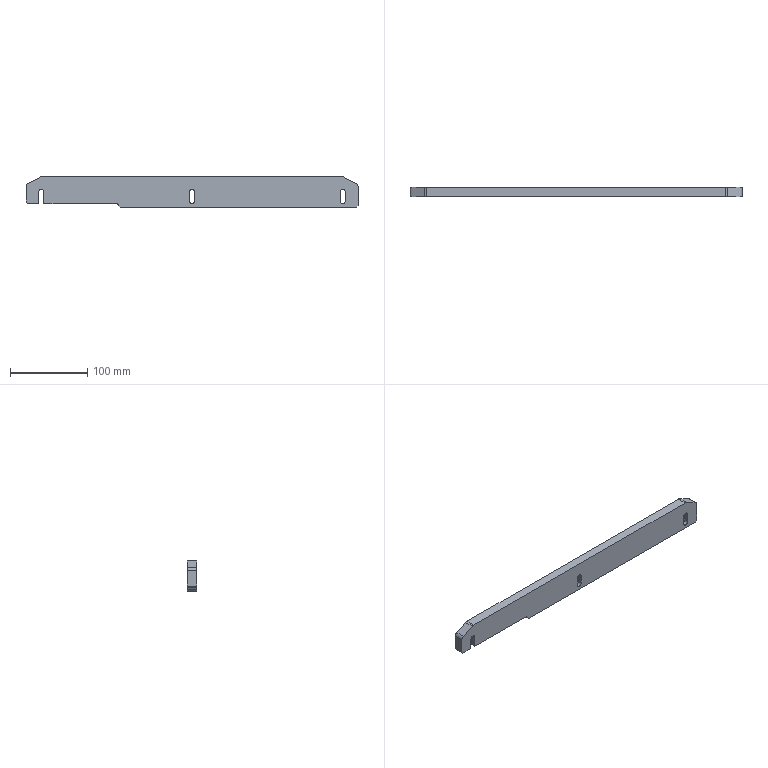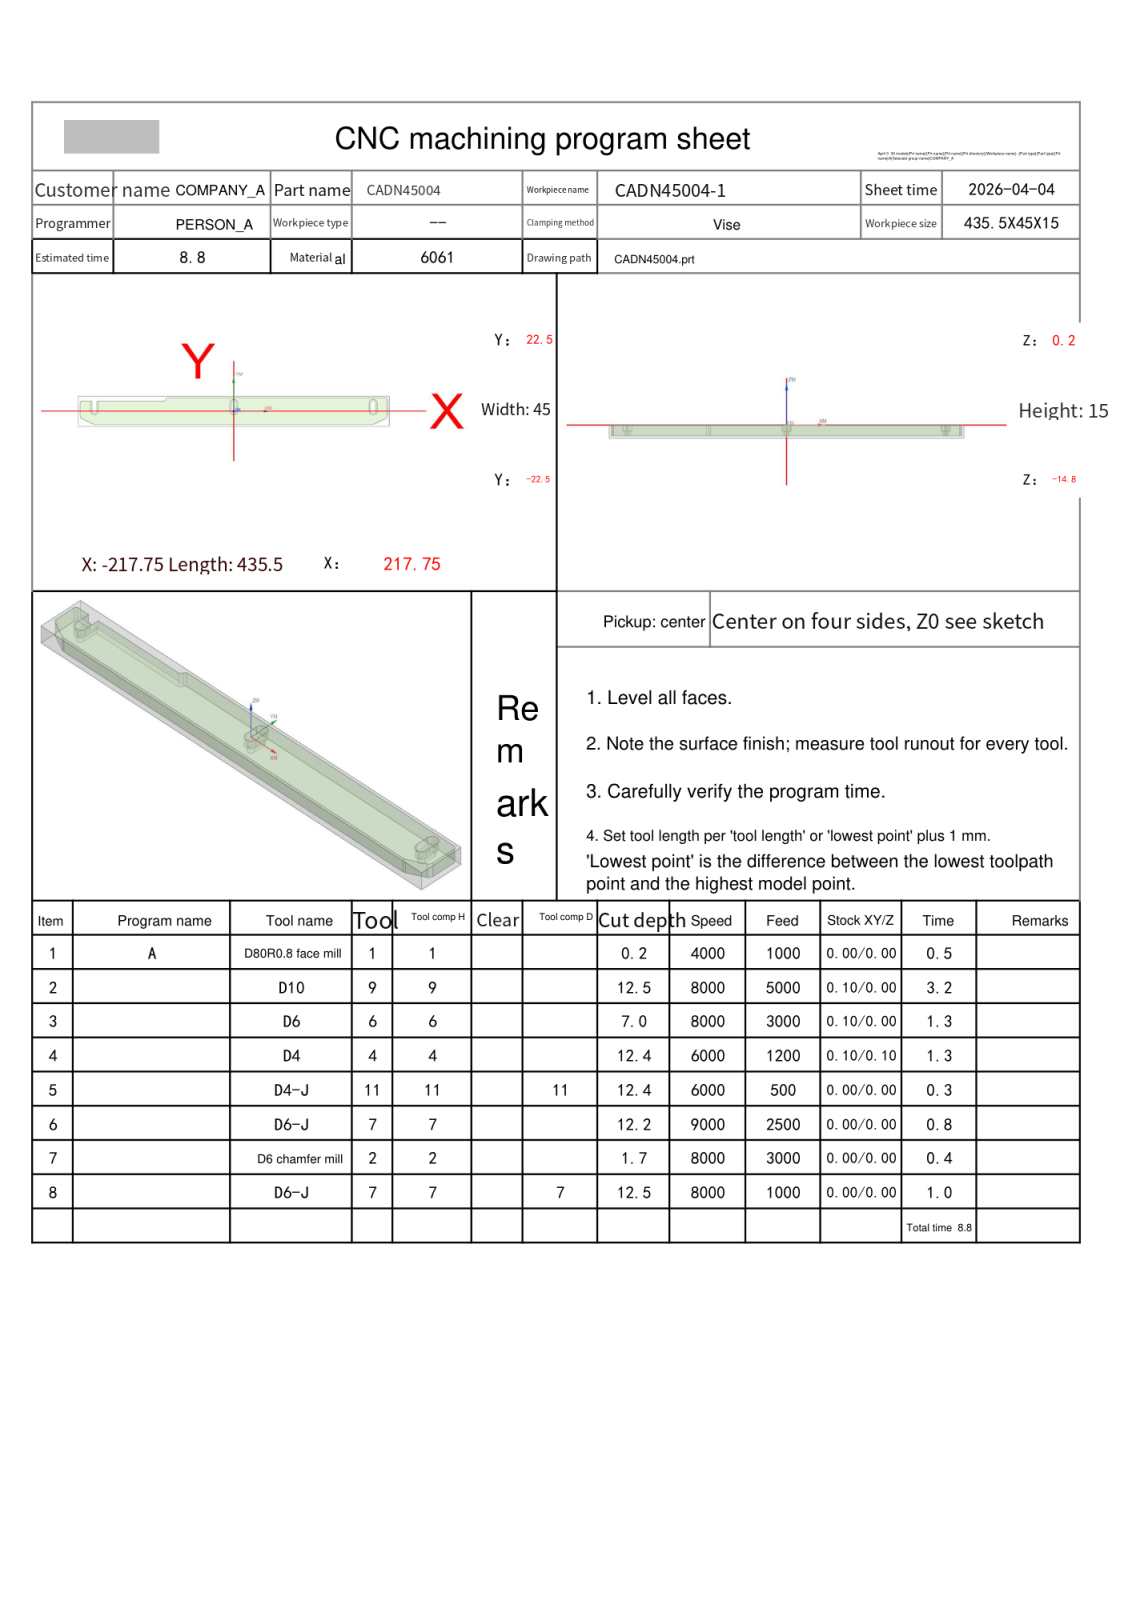NC program | NX | posted by the shop | part box 430.5 x 12 x 40 mm
Lines 1 to 1346 of 3420, first 1256 of 1344 lines:
%
O0001
(Machine time: 10.58 MIN)
(===Total Tool:7===)
(T1=D80R0.8 face mill D=80.  R=0.8  D-  H01 Z=-0.   )
(T9=D10     D=10.  R=0.   D-  H09 Z=-12.3 )
(T6=D6      D=6.   R=0.   D-  H06 Z=-6.8  )
(T4=D4      D=4.   R=0.   D-  H04 Z=-12.2 )
(T11=D4-J   D=4.   R=0.   D11 H11 Z=-12.2 )
(T7=D6-J    D=6.   R=0.   D7  H07 Z=-12.3 )
(T2=D6 chamfer mill   D=6.   R=0.   D-  H02 Z=-1.5  )
G80 G90 G17 G49 G40
G91 G28 Z0
M01
N1 T01 M06
(D80R0.8 face mill  D=80. R=0.8 H=01 ce=0.00 di=0.00)
G00 G90 G54 X260.25 Y0.0 M03 S4000
G43 H01 Z20.
M08
Z2.
G01 Z0.0 F1000.
X255.25
X-255.25
X-260.25
Z2.
G00 Z20.
G91 G28 Z0.0
M05
M09
G91 G28 Z0.0
M01
N2 T09 M06
(D10  D=10. R=0. H=09 ce=0.10 di=0.00)
G00 G90 G54 X0.0 Y-25.1 M03 S8000
G43 H09 Z20.
M08
Z.5
G01 X-194.07 Z.337 F5000.
G02 X-198.587 Y-24.034 Z.333 I0.0 J10.1
G01 X-214.767 Y-15.944 Z.318
G02 X-220.35 Y-6.91 Z.308 I4.517 J9.034
G01 Y13. Z.292
G02 X-218.856 Y16.606 Z.288 I5.1 J0.0
G01 X-216.856 Y18.606 Z.286
G02 X-213.25 Y20.1 Z.282 I3.606 J-3.606
G01 X-198.55 Z.27
G02 X-195.25 Y18.888 Z.267 I0.0 J-5.1
X-191.95 Y20.1 Z.264 I3.3 J-3.888
G01 X-99.898 Z.187
G02 X-98.856 Y21.606 Z.185 I4.648 J-2.1
G01 X-96.856 Y23.606 Z.183
G02 X-93.25 Y25.1 Z.179 I3.606 J-3.606
G01 X213.25 Z-.078
G02 X216.856 Y23.606 Z-.082 I0.0 J-5.1
G01 X218.856 Y21.606 Z-.084
G02 X220.35 Y18. Z-.087 I-3.606 J-3.606
G01 Y-6.91 Z-.108
G02 X214.767 Y-15.944 Z-.118 I-10.1 J0.0
G01 X198.587 Y-24.034 Z-.133
G02 X194.07 Y-25.1 Z-.137 I-4.517 J9.034
G01 X-194.07 Z-.463
G02 X-198.587 Y-24.034 Z-.467 I0.0 J10.1
G01 X-214.767 Y-15.944 Z-.482
G02 X-220.35 Y-6.91 Z-.492 I4.517 J9.034
G01 Y13. Z-.508
G02 X-218.856 Y16.606 Z-.512 I5.1 J0.0
G01 X-216.856 Y18.606 Z-.514
G02 X-213.25 Y20.1 Z-.518 I3.606 J-3.606
G01 X-198.55 Z-.53
G02 X-195.25 Y18.888 Z-.533 I0.0 J-5.1
X-191.95 Y20.1 Z-.536 I3.3 J-3.888
G01 X-99.898 Z-.613
G02 X-98.856 Y21.606 Z-.615 I4.648 J-2.1
G01 X-96.856 Y23.606 Z-.617
G02 X-93.25 Y25.1 Z-.621 I3.606 J-3.606
G01 X213.25 Z-.878
G02 X216.856 Y23.606 Z-.882 I0.0 J-5.1
G01 X218.856 Y21.606 Z-.884
G02 X220.35 Y18. Z-.887 I-3.606 J-3.606
G01 Y-6.91 Z-.908
G02 X214.767 Y-15.944 Z-.918 I-10.1 J0.0
G01 X198.587 Y-24.034 Z-.933
G02 X194.07 Y-25.1 Z-.937 I-4.517 J9.034
G01 X-194.07 Z-1.263
G02 X-198.587 Y-24.034 Z-1.267 I0.0 J10.1
G01 X-214.767 Y-15.944 Z-1.282
G02 X-220.35 Y-6.91 Z-1.292 I4.517 J9.034
G01 Y13. Z-1.308
G02 X-218.856 Y16.606 Z-1.312 I5.1 J0.0
G01 X-216.856 Y18.606 Z-1.314
G02 X-213.25 Y20.1 Z-1.318 I3.606 J-3.606
G01 X-198.55 Z-1.33
G02 X-195.25 Y18.888 Z-1.333 I0.0 J-5.1
X-191.95 Y20.1 Z-1.336 I3.3 J-3.888
G01 X-99.898 Z-1.413
G02 X-98.856 Y21.606 Z-1.415 I4.648 J-2.1
G01 X-96.856 Y23.606 Z-1.417
G02 X-93.25 Y25.1 Z-1.421 I3.606 J-3.606
G01 X213.25 Z-1.678
G02 X216.856 Y23.606 Z-1.682 I0.0 J-5.1
G01 X218.856 Y21.606 Z-1.684
G02 X220.35 Y18. Z-1.687 I-3.606 J-3.606
G01 Y-6.91 Z-1.708
G02 X214.767 Y-15.944 Z-1.718 I-10.1 J0.0
G01 X198.587 Y-24.034 Z-1.733
G02 X194.07 Y-25.1 Z-1.737 I-4.517 J9.034
G01 X-194.07 Z-2.063
G02 X-198.587 Y-24.034 Z-2.067 I0.0 J10.1
G01 X-214.767 Y-15.944 Z-2.082
G02 X-220.35 Y-6.91 Z-2.092 I4.517 J9.034
G01 Y13. Z-2.108
G02 X-218.856 Y16.606 Z-2.112 I5.1 J0.0
G01 X-216.856 Y18.606 Z-2.114
G02 X-213.25 Y20.1 Z-2.118 I3.606 J-3.606
G01 X-198.55 Z-2.13
G02 X-195.25 Y18.888 Z-2.133 I0.0 J-5.1
X-191.95 Y20.1 Z-2.136 I3.3 J-3.888
G01 X-99.898 Z-2.213
G02 X-98.856 Y21.606 Z-2.215 I4.648 J-2.1
G01 X-96.856 Y23.606 Z-2.217
G02 X-93.25 Y25.1 Z-2.221 I3.606 J-3.606
G01 X213.25 Z-2.478
G02 X216.856 Y23.606 Z-2.482 I0.0 J-5.1
G01 X218.856 Y21.606 Z-2.484
G02 X220.35 Y18. Z-2.487 I-3.606 J-3.606
G01 Y-6.91 Z-2.508
G02 X214.767 Y-15.944 Z-2.518 I-10.1 J0.0
G01 X198.587 Y-24.034 Z-2.533
G02 X194.07 Y-25.1 Z-2.537 I-4.517 J9.034
G01 X-194.07 Z-2.863
G02 X-198.587 Y-24.034 Z-2.867 I0.0 J10.1
G01 X-214.767 Y-15.944 Z-2.882
G02 X-220.35 Y-6.91 Z-2.892 I4.517 J9.034
G01 Y13. Z-2.908
G02 X-218.856 Y16.606 Z-2.912 I5.1 J0.0
G01 X-216.856 Y18.606 Z-2.914
G02 X-213.25 Y20.1 Z-2.918 I3.606 J-3.606
G01 X-198.55 Z-2.93
G02 X-195.25 Y18.888 Z-2.933 I0.0 J-5.1
X-191.95 Y20.1 Z-2.936 I3.3 J-3.888
G01 X-99.898 Z-3.013
G02 X-98.856 Y21.606 Z-3.015 I4.648 J-2.1
G01 X-96.856 Y23.606 Z-3.017
G02 X-93.25 Y25.1 Z-3.021 I3.606 J-3.606
G01 X213.25 Z-3.278
G02 X216.856 Y23.606 Z-3.282 I0.0 J-5.1
G01 X218.856 Y21.606 Z-3.284
G02 X220.35 Y18. Z-3.287 I-3.606 J-3.606
G01 Y-6.91 Z-3.308
G02 X214.767 Y-15.944 Z-3.318 I-10.1 J0.0
G01 X198.587 Y-24.034 Z-3.333
G02 X194.07 Y-25.1 Z-3.337 I-4.517 J9.034
G01 X-194.07 Z-3.663
G02 X-198.587 Y-24.034 Z-3.667 I0.0 J10.1
G01 X-214.767 Y-15.944 Z-3.682
G02 X-220.35 Y-6.91 Z-3.692 I4.517 J9.034
G01 Y13. Z-3.708
G02 X-218.856 Y16.606 Z-3.712 I5.1 J0.0
G01 X-216.856 Y18.606 Z-3.714
G02 X-213.25 Y20.1 Z-3.718 I3.606 J-3.606
G01 X-198.55 Z-3.73
G02 X-195.25 Y18.888 Z-3.733 I0.0 J-5.1
X-191.95 Y20.1 Z-3.736 I3.3 J-3.888
G01 X-99.898 Z-3.813
G02 X-98.856 Y21.606 Z-3.815 I4.648 J-2.1
G01 X-96.856 Y23.606 Z-3.817
G02 X-93.25 Y25.1 Z-3.821 I3.606 J-3.606
G01 X213.25 Z-4.078
G02 X216.856 Y23.606 Z-4.082 I0.0 J-5.1
G01 X218.856 Y21.606 Z-4.084
G02 X220.35 Y18. Z-4.087 I-3.606 J-3.606
G01 Y-6.91 Z-4.108
G02 X214.767 Y-15.944 Z-4.118 I-10.1 J0.0
G01 X198.587 Y-24.034 Z-4.133
G02 X194.07 Y-25.1 Z-4.137 I-4.517 J9.034
G01 X-194.07 Z-4.463
G02 X-198.587 Y-24.034 Z-4.467 I0.0 J10.1
G01 X-214.767 Y-15.944 Z-4.482
G02 X-220.35 Y-6.91 Z-4.492 I4.517 J9.034
G01 Y13. Z-4.508
G02 X-218.856 Y16.606 Z-4.512 I5.1 J0.0
G01 X-216.856 Y18.606 Z-4.514
G02 X-213.25 Y20.1 Z-4.518 I3.606 J-3.606
G01 X-198.55 Z-4.53
G02 X-195.25 Y18.888 Z-4.533 I0.0 J-5.1
X-191.95 Y20.1 Z-4.536 I3.3 J-3.888
G01 X-99.898 Z-4.613
G02 X-98.856 Y21.606 Z-4.615 I4.648 J-2.1
G01 X-96.856 Y23.606 Z-4.617
G02 X-93.25 Y25.1 Z-4.621 I3.606 J-3.606
G01 X213.25 Z-4.878
G02 X216.856 Y23.606 Z-4.882 I0.0 J-5.1
G01 X218.856 Y21.606 Z-4.884
G02 X220.35 Y18. Z-4.887 I-3.606 J-3.606
G01 Y-6.91 Z-4.908
G02 X214.767 Y-15.944 Z-4.918 I-10.1 J0.0
G01 X198.587 Y-24.034 Z-4.933
G02 X194.07 Y-25.1 Z-4.937 I-4.517 J9.034
G01 X-194.07 Z-5.263
G02 X-198.587 Y-24.034 Z-5.267 I0.0 J10.1
G01 X-214.767 Y-15.944 Z-5.282
G02 X-220.35 Y-6.91 Z-5.292 I4.517 J9.034
G01 Y13. Z-5.308
G02 X-218.856 Y16.606 Z-5.312 I5.1 J0.0
G01 X-216.856 Y18.606 Z-5.314
G02 X-213.25 Y20.1 Z-5.318 I3.606 J-3.606
G01 X-198.55 Z-5.33
G02 X-195.25 Y18.888 Z-5.333 I0.0 J-5.1
X-191.95 Y20.1 Z-5.336 I3.3 J-3.888
G01 X-99.898 Z-5.413
G02 X-98.856 Y21.606 Z-5.415 I4.648 J-2.1
G01 X-96.856 Y23.606 Z-5.417
G02 X-93.25 Y25.1 Z-5.421 I3.606 J-3.606
G01 X213.25 Z-5.678
G02 X216.856 Y23.606 Z-5.682 I0.0 J-5.1
G01 X218.856 Y21.606 Z-5.684
G02 X220.35 Y18. Z-5.687 I-3.606 J-3.606
G01 Y-6.91 Z-5.708
G02 X214.767 Y-15.944 Z-5.718 I-10.1 J0.0
G01 X198.587 Y-24.034 Z-5.733
G02 X194.07 Y-25.1 Z-5.737 I-4.517 J9.034
G01 X-194.07 Z-6.063
G02 X-198.587 Y-24.034 Z-6.067 I0.0 J10.1
G01 X-214.767 Y-15.944 Z-6.082
G02 X-220.35 Y-6.91 Z-6.092 I4.517 J9.034
G01 Y13. Z-6.108
G02 X-218.856 Y16.606 Z-6.112 I5.1 J0.0
G01 X-216.856 Y18.606 Z-6.114
G02 X-213.25 Y20.1 Z-6.118 I3.606 J-3.606
G01 X-198.55 Z-6.13
G02 X-195.25 Y18.888 Z-6.133 I0.0 J-5.1
X-191.95 Y20.1 Z-6.136 I3.3 J-3.888
G01 X-99.898 Z-6.213
G02 X-98.856 Y21.606 Z-6.215 I4.648 J-2.1
G01 X-96.856 Y23.606 Z-6.217
G02 X-93.25 Y25.1 Z-6.221 I3.606 J-3.606
G01 X213.25 Z-6.478
G02 X216.856 Y23.606 Z-6.482 I0.0 J-5.1
G01 X218.856 Y21.606 Z-6.484
G02 X220.35 Y18. Z-6.487 I-3.606 J-3.606
G01 Y-6.91 Z-6.508
G02 X214.767 Y-15.944 Z-6.518 I-10.1 J0.0
G01 X198.587 Y-24.034 Z-6.533
G02 X194.07 Y-25.1 Z-6.537 I-4.517 J9.034
G01 X-194.07 Z-6.863
G02 X-198.587 Y-24.034 Z-6.867 I0.0 J10.1
G01 X-214.767 Y-15.944 Z-6.882
G02 X-220.35 Y-6.91 Z-6.892 I4.517 J9.034
G01 Y13. Z-6.908
G02 X-218.856 Y16.606 Z-6.912 I5.1 J0.0
G01 X-216.856 Y18.606 Z-6.914
G02 X-213.25 Y20.1 Z-6.918 I3.606 J-3.606
G01 X-198.55 Z-6.93
G02 X-195.25 Y18.888 Z-6.933 I0.0 J-5.1
X-191.95 Y20.1 Z-6.936 I3.3 J-3.888
G01 X-99.898 Z-7.013
G02 X-98.856 Y21.606 Z-7.015 I4.648 J-2.1
G01 X-96.856 Y23.606 Z-7.017
G02 X-93.25 Y25.1 Z-7.021 I3.606 J-3.606
G01 X213.25 Z-7.278
G02 X216.856 Y23.606 Z-7.282 I0.0 J-5.1
G01 X218.856 Y21.606 Z-7.284
G02 X220.35 Y18. Z-7.287 I-3.606 J-3.606
G01 Y-6.91 Z-7.308
G02 X214.767 Y-15.944 Z-7.318 I-10.1 J0.0
G01 X198.587 Y-24.034 Z-7.333
G02 X194.07 Y-25.1 Z-7.337 I-4.517 J9.034
G01 X-194.07 Z-7.663
G02 X-198.587 Y-24.034 Z-7.667 I0.0 J10.1
G01 X-214.767 Y-15.944 Z-7.682
G02 X-220.35 Y-6.91 Z-7.692 I4.517 J9.034
G01 Y13. Z-7.708
G02 X-218.856 Y16.606 Z-7.712 I5.1 J0.0
G01 X-216.856 Y18.606 Z-7.714
G02 X-213.25 Y20.1 Z-7.718 I3.606 J-3.606
G01 X-198.55 Z-7.73
G02 X-195.25 Y18.888 Z-7.733 I0.0 J-5.1
X-191.95 Y20.1 Z-7.736 I3.3 J-3.888
G01 X-99.898 Z-7.813
G02 X-98.856 Y21.606 Z-7.815 I4.648 J-2.1
G01 X-96.856 Y23.606 Z-7.817
G02 X-93.25 Y25.1 Z-7.821 I3.606 J-3.606
G01 X213.25 Z-8.078
G02 X216.856 Y23.606 Z-8.082 I0.0 J-5.1
G01 X218.856 Y21.606 Z-8.084
G02 X220.35 Y18. Z-8.087 I-3.606 J-3.606
G01 Y-6.91 Z-8.108
G02 X214.767 Y-15.944 Z-8.118 I-10.1 J0.0
G01 X198.587 Y-24.034 Z-8.133
G02 X194.07 Y-25.1 Z-8.137 I-4.517 J9.034
G01 X-194.07 Z-8.463
G02 X-198.587 Y-24.034 Z-8.467 I0.0 J10.1
G01 X-214.767 Y-15.944 Z-8.482
G02 X-220.35 Y-6.91 Z-8.492 I4.517 J9.034
G01 Y13. Z-8.508
G02 X-218.856 Y16.606 Z-8.512 I5.1 J0.0
G01 X-216.856 Y18.606 Z-8.514
G02 X-213.25 Y20.1 Z-8.518 I3.606 J-3.606
G01 X-198.55 Z-8.53
G02 X-195.25 Y18.888 Z-8.533 I0.0 J-5.1
X-191.95 Y20.1 Z-8.536 I3.3 J-3.888
G01 X-99.898 Z-8.613
G02 X-98.856 Y21.606 Z-8.615 I4.648 J-2.1
G01 X-96.856 Y23.606 Z-8.617
G02 X-93.25 Y25.1 Z-8.621 I3.606 J-3.606
G01 X213.25 Z-8.878
G02 X216.856 Y23.606 Z-8.882 I0.0 J-5.1
G01 X218.856 Y21.606 Z-8.884
G02 X220.35 Y18. Z-8.887 I-3.606 J-3.606
G01 Y-6.91 Z-8.908
G02 X214.767 Y-15.944 Z-8.918 I-10.1 J0.0
G01 X198.587 Y-24.034 Z-8.933
G02 X194.07 Y-25.1 Z-8.937 I-4.517 J9.034
G01 X-194.07 Z-9.263
G02 X-198.587 Y-24.034 Z-9.267 I0.0 J10.1
G01 X-214.767 Y-15.944 Z-9.282
G02 X-220.35 Y-6.91 Z-9.292 I4.517 J9.034
G01 Y13. Z-9.308
G02 X-218.856 Y16.606 Z-9.312 I5.1 J0.0
G01 X-216.856 Y18.606 Z-9.314
G02 X-213.25 Y20.1 Z-9.318 I3.606 J-3.606
G01 X-198.55 Z-9.33
G02 X-195.25 Y18.888 Z-9.333 I0.0 J-5.1
X-191.95 Y20.1 Z-9.336 I3.3 J-3.888
G01 X-99.898 Z-9.413
G02 X-98.856 Y21.606 Z-9.415 I4.648 J-2.1
G01 X-96.856 Y23.606 Z-9.417
G02 X-93.25 Y25.1 Z-9.421 I3.606 J-3.606
G01 X213.25 Z-9.678
G02 X216.856 Y23.606 Z-9.682 I0.0 J-5.1
G01 X218.856 Y21.606 Z-9.684
G02 X220.35 Y18. Z-9.687 I-3.606 J-3.606
G01 Y-6.91 Z-9.708
G02 X214.767 Y-15.944 Z-9.718 I-10.1 J0.0
G01 X198.587 Y-24.034 Z-9.733
G02 X194.07 Y-25.1 Z-9.737 I-4.517 J9.034
G01 X-194.07 Z-10.063
G02 X-198.587 Y-24.034 Z-10.067 I0.0 J10.1
G01 X-214.767 Y-15.944 Z-10.082
G02 X-220.35 Y-6.91 Z-10.092 I4.517 J9.034
G01 Y13. Z-10.108
G02 X-218.856 Y16.606 Z-10.112 I5.1 J0.0
G01 X-216.856 Y18.606 Z-10.114
G02 X-213.25 Y20.1 Z-10.118 I3.606 J-3.606
G01 X-198.55 Z-10.13
G02 X-195.25 Y18.888 Z-10.133 I0.0 J-5.1
X-191.95 Y20.1 Z-10.136 I3.3 J-3.888
G01 X-99.898 Z-10.213
G02 X-98.856 Y21.606 Z-10.215 I4.648 J-2.1
G01 X-96.856 Y23.606 Z-10.217
G02 X-93.25 Y25.1 Z-10.221 I3.606 J-3.606
G01 X213.25 Z-10.478
G02 X216.856 Y23.606 Z-10.482 I0.0 J-5.1
G01 X218.856 Y21.606 Z-10.484
G02 X220.35 Y18. Z-10.487 I-3.606 J-3.606
G01 Y-6.91 Z-10.508
G02 X214.767 Y-15.944 Z-10.518 I-10.1 J0.0
G01 X198.587 Y-24.034 Z-10.533
G02 X194.07 Y-25.1 Z-10.537 I-4.517 J9.034
G01 X-194.07 Z-10.863
G02 X-198.587 Y-24.034 Z-10.867 I0.0 J10.1
G01 X-214.767 Y-15.944 Z-10.882
G02 X-220.35 Y-6.91 Z-10.892 I4.517 J9.034
G01 Y13. Z-10.908
G02 X-218.856 Y16.606 Z-10.912 I5.1 J0.0
G01 X-216.856 Y18.606 Z-10.914
G02 X-213.25 Y20.1 Z-10.918 I3.606 J-3.606
G01 X-198.55 Z-10.93
G02 X-195.25 Y18.888 Z-10.933 I0.0 J-5.1
X-191.95 Y20.1 Z-10.936 I3.3 J-3.888
G01 X-99.898 Z-11.013
G02 X-98.856 Y21.606 Z-11.015 I4.648 J-2.1
G01 X-96.856 Y23.606 Z-11.017
G02 X-93.25 Y25.1 Z-11.021 I3.606 J-3.606
G01 X213.25 Z-11.278
G02 X216.856 Y23.606 Z-11.282 I0.0 J-5.1
G01 X218.856 Y21.606 Z-11.284
G02 X220.35 Y18. Z-11.287 I-3.606 J-3.606
G01 Y-6.91 Z-11.308
G02 X214.767 Y-15.944 Z-11.318 I-10.1 J0.0
G01 X198.587 Y-24.034 Z-11.333
G02 X194.07 Y-25.1 Z-11.337 I-4.517 J9.034
G01 X-194.07 Z-11.663
G02 X-198.587 Y-24.034 Z-11.667 I0.0 J10.1
G01 X-214.767 Y-15.944 Z-11.682
G02 X-220.35 Y-6.91 Z-11.692 I4.517 J9.034
G01 Y13. Z-11.708
G02 X-218.856 Y16.606 Z-11.712 I5.1 J0.0
G01 X-216.856 Y18.606 Z-11.714
G02 X-213.25 Y20.1 Z-11.718 I3.606 J-3.606
G01 X-198.55 Z-11.73
G02 X-195.25 Y18.888 Z-11.733 I0.0 J-5.1
X-191.95 Y20.1 Z-11.736 I3.3 J-3.888
G01 X-99.898 Z-11.813
G02 X-98.856 Y21.606 Z-11.815 I4.648 J-2.1
G01 X-96.856 Y23.606 Z-11.817
G02 X-93.25 Y25.1 Z-11.821 I3.606 J-3.606
G01 X213.25 Z-12.078
G02 X216.856 Y23.606 Z-12.082 I0.0 J-5.1
G01 X218.856 Y21.606 Z-12.084
G02 X220.35 Y18. Z-12.087 I-3.606 J-3.606
G01 Y-6.91 Z-12.108
G02 X214.767 Y-15.944 Z-12.118 I-10.1 J0.0
G01 X198.587 Y-24.034 Z-12.133
G02 X194.07 Y-25.1 Z-12.137 I-4.517 J9.034
G01 X0.0 Z-12.3
X-194.07
G02 X-198.587 Y-24.034 I0.0 J10.1
G01 X-214.767 Y-15.944
G02 X-220.35 Y-6.91 I4.517 J9.034
G01 Y13.
G02 X-218.856 Y16.606 I5.1 J0.0
G01 X-216.856 Y18.606
G02 X-213.25 Y20.1 I3.606 J-3.606
G01 X-198.55
G02 X-195.25 Y18.888 I0.0 J-5.1
X-191.95 Y20.1 I3.3 J-3.888
G01 X-99.898
G02 X-98.856 Y21.606 I4.648 J-2.1
G01 X-96.856 Y23.606
G02 X-93.25 Y25.1 I3.606 J-3.606
G01 X213.25
G02 X216.856 Y23.606 I0.0 J-5.1
G01 X218.856 Y21.606
G02 X220.35 Y18. I-3.606 J-3.606
G01 Y-6.91
G02 X214.767 Y-15.944 I-10.1 J0.0
G01 X198.587 Y-24.034
G02 X194.07 Y-25.1 I-4.517 J9.034
G01 X0.0
X-.5
Z-11.3
G00 Z20.
G91 G28 Z0.0
M05
M09
G91 G28 Z0.0
M01
N3 T06 M06
(D6  D=6. R=0. H=06 ce=0.10 di=0.00)
G00 G90 G54 X-2.4 Y6. M03 S6000
G43 H06 Z20.
M08
Z.5
G01 Y0.0 Z.455 F2000.
G03 X0.0 Y-2.4 Z.427 I2.4 J0.0
X2.4 Y0.0 Z.399 I0.0 J2.4
G01 Y12. Z.309
G03 X0.0 Y14.4 Z.281 I-2.4 J0.0
X-2.4 Y12. Z.253 I0.0 J-2.4
G01 Y0.0 Z.163
G03 X0.0 Y-2.4 Z.135 I2.4 J0.0
X2.4 Y0.0 Z.107 I0.0 J2.4
G01 Y12. Z.017
G03 X0.0 Y14.4 Z-.011 I-2.4 J0.0
X-2.4 Y12. Z-.039 I0.0 J-2.4
G01 Y0.0 Z-.129
G03 X0.0 Y-2.4 Z-.157 I2.4 J0.0
X2.4 Y0.0 Z-.185 I0.0 J2.4
G01 Y12. Z-.275
G03 X0.0 Y14.4 Z-.303 I-2.4 J0.0
X-2.4 Y12. Z-.331 I0.0 J-2.4
G01 Y0.0 Z-.421
G03 X0.0 Y-2.4 Z-.449 I2.4 J0.0
X2.4 Y0.0 Z-.477 I0.0 J2.4
G01 Y12. Z-.567
G03 X0.0 Y14.4 Z-.595 I-2.4 J0.0
X-2.4 Y12. Z-.623 I0.0 J-2.4
G01 Y0.0 Z-.713
G03 X0.0 Y-2.4 Z-.741 I2.4 J0.0
X2.4 Y0.0 Z-.769 I0.0 J2.4
G01 Y12. Z-.859
G03 X0.0 Y14.4 Z-.887 I-2.4 J0.0
X-2.4 Y12. Z-.915 I0.0 J-2.4
G01 Y0.0 Z-1.005
G03 X0.0 Y-2.4 Z-1.033 I2.4 J0.0
X2.4 Y0.0 Z-1.061 I0.0 J2.4
G01 Y12. Z-1.151
G03 X0.0 Y14.4 Z-1.179 I-2.4 J0.0
X-2.4 Y12. Z-1.207 I0.0 J-2.4
G01 Y0.0 Z-1.297
G03 X0.0 Y-2.4 Z-1.325 I2.4 J0.0
X2.4 Y0.0 Z-1.353 I0.0 J2.4
G01 Y12. Z-1.443
G03 X0.0 Y14.4 Z-1.471 I-2.4 J0.0
X-2.4 Y12. Z-1.499 I0.0 J-2.4
G01 Y0.0 Z-1.589
G03 X0.0 Y-2.4 Z-1.617 I2.4 J0.0
X2.4 Y0.0 Z-1.645 I0.0 J2.4
G01 Y12. Z-1.735
G03 X0.0 Y14.4 Z-1.763 I-2.4 J0.0
X-2.4 Y12. Z-1.791 I0.0 J-2.4
G01 Y0.0 Z-1.881
G03 X0.0 Y-2.4 Z-1.909 I2.4 J0.0
X2.4 Y0.0 Z-1.937 I0.0 J2.4
G01 Y12. Z-2.027
G03 X0.0 Y14.4 Z-2.055 I-2.4 J0.0
X-2.4 Y12. Z-2.083 I0.0 J-2.4
G01 Y0.0 Z-2.173
G03 X0.0 Y-2.4 Z-2.201 I2.4 J0.0
X2.4 Y0.0 Z-2.229 I0.0 J2.4
G01 Y12. Z-2.319
G03 X0.0 Y14.4 Z-2.347 I-2.4 J0.0
X-2.4 Y12. Z-2.375 I0.0 J-2.4
G01 Y0.0 Z-2.465
G03 X0.0 Y-2.4 Z-2.493 I2.4 J0.0
X2.4 Y0.0 Z-2.521 I0.0 J2.4
G01 Y12. Z-2.611
G03 X0.0 Y14.4 Z-2.639 I-2.4 J0.0
X-2.4 Y12. Z-2.667 I0.0 J-2.4
G01 Y0.0 Z-2.757
G03 X0.0 Y-2.4 Z-2.785 I2.4 J0.0
X2.4 Y0.0 Z-2.813 I0.0 J2.4
G01 Y12. Z-2.903
G03 X0.0 Y14.4 Z-2.931 I-2.4 J0.0
X-2.4 Y12. Z-2.959 I0.0 J-2.4
G01 Y0.0 Z-3.049
G03 X0.0 Y-2.4 Z-3.077 I2.4 J0.0
X2.4 Y0.0 Z-3.105 I0.0 J2.4
G01 Y12. Z-3.195
G03 X0.0 Y14.4 Z-3.223 I-2.4 J0.0
X-2.4 Y12. Z-3.251 I0.0 J-2.4
G01 Y0.0 Z-3.341
G03 X0.0 Y-2.4 Z-3.369 I2.4 J0.0
X2.4 Y0.0 Z-3.397 I0.0 J2.4
G01 Y12. Z-3.487
G03 X0.0 Y14.4 Z-3.515 I-2.4 J0.0
X-2.4 Y12. Z-3.543 I0.0 J-2.4
G01 Y0.0 Z-3.633
G03 X0.0 Y-2.4 Z-3.661 I2.4 J0.0
X2.4 Y0.0 Z-3.689 I0.0 J2.4
G01 Y12. Z-3.779
G03 X0.0 Y14.4 Z-3.807 I-2.4 J0.0
X-2.4 Y12. Z-3.835 I0.0 J-2.4
G01 Y0.0 Z-3.925
G03 X0.0 Y-2.4 Z-3.953 I2.4 J0.0
X2.4 Y0.0 Z-3.981 I0.0 J2.4
G01 Y12. Z-4.071
G03 X0.0 Y14.4 Z-4.099 I-2.4 J0.0
X-2.4 Y12. Z-4.127 I0.0 J-2.4
G01 Y0.0 Z-4.217
G03 X0.0 Y-2.4 Z-4.245 I2.4 J0.0
X2.4 Y0.0 Z-4.273 I0.0 J2.4
G01 Y12. Z-4.363
G03 X0.0 Y14.4 Z-4.391 I-2.4 J0.0
X-2.4 Y12. Z-4.419 I0.0 J-2.4
G01 Y0.0 Z-4.509
G03 X0.0 Y-2.4 Z-4.537 I2.4 J0.0
X2.4 Y0.0 Z-4.565 I0.0 J2.4
G01 Y12. Z-4.655
G03 X0.0 Y14.4 Z-4.683 I-2.4 J0.0
X-2.4 Y12. Z-4.711 I0.0 J-2.4
G01 Y0.0 Z-4.801
G03 X0.0 Y-2.4 Z-4.829 I2.4 J0.0
X2.4 Y0.0 Z-4.857 I0.0 J2.4
G01 Y12. Z-4.947
G03 X0.0 Y14.4 Z-4.975 I-2.4 J0.0
X-2.4 Y12. Z-5.003 I0.0 J-2.4
G01 Y0.0 Z-5.093
G03 X0.0 Y-2.4 Z-5.121 I2.4 J0.0
X2.4 Y0.0 Z-5.149 I0.0 J2.4
G01 Y12. Z-5.239
G03 X0.0 Y14.4 Z-5.267 I-2.4 J0.0
X-2.4 Y12. Z-5.295 I0.0 J-2.4
G01 Y0.0 Z-5.385
G03 X0.0 Y-2.4 Z-5.413 I2.4 J0.0
X2.4 Y0.0 Z-5.441 I0.0 J2.4
G01 Y12. Z-5.531
G03 X0.0 Y14.4 Z-5.559 I-2.4 J0.0
X-2.4 Y12. Z-5.587 I0.0 J-2.4
G01 Y0.0 Z-5.677
G03 X0.0 Y-2.4 Z-5.705 I2.4 J0.0
X2.4 Y0.0 Z-5.733 I0.0 J2.4
G01 Y12. Z-5.823
G03 X0.0 Y14.4 Z-5.851 I-2.4 J0.0
X-2.4 Y12. Z-5.879 I0.0 J-2.4
G01 Y0.0 Z-5.969
G03 X0.0 Y-2.4 Z-5.997 I2.4 J0.0
X2.4 Y0.0 Z-6.025 I0.0 J2.4
G01 Y12. Z-6.115
G03 X0.0 Y14.4 Z-6.143 I-2.4 J0.0
X-2.4 Y12. Z-6.171 I0.0 J-2.4
G01 Y0.0 Z-6.261
G03 X0.0 Y-2.4 Z-6.289 I2.4 J0.0
X2.4 Y0.0 Z-6.317 I0.0 J2.4
G01 Y12. Z-6.407
G03 X0.0 Y14.4 Z-6.435 I-2.4 J0.0
X-2.4 Y12. Z-6.463 I0.0 J-2.4
G01 Y0.0 Z-6.553
G03 X0.0 Y-2.4 Z-6.581 I2.4 J0.0
X2.4 Y0.0 Z-6.609 I0.0 J2.4
G01 Y12. Z-6.699
G03 X0.0 Y14.4 Z-6.727 I-2.4 J0.0
X-2.4 Y12. Z-6.755 I0.0 J-2.4
G01 Y6. Z-6.8
Y0.0
G03 X0.0 Y-2.4 I2.4 J0.0
X2.4 Y0.0 I0.0 J2.4
G01 Y12.
G03 X0.0 Y14.4 I-2.4 J0.0
X-2.4 Y12. I0.0 J-2.4
G01 Y6.
Y5.5
Z-5.8
G00 Z20.
X192.85 Y6.
Z.5
G01 Y0.0 Z.455
G03 X193.423 Y-1.557 Z.443 I2.4 J0.0
X195.25 Y-2.4 Z.427 I1.827 J1.557
X197.65 Y0.0 Z.399 I0.0 J2.4
G01 Y12. Z.309
G03 X195.25 Y14.4 Z.281 I-2.4 J0.0
X192.85 Y12. Z.253 I0.0 J-2.4
G01 Y0.0 Z.163
G03 X193.423 Y-1.557 Z.151 I2.4 J0.0
X195.25 Y-2.4 Z.135 I1.827 J1.557
X197.65 Y0.0 Z.107 I0.0 J2.4
G01 Y12. Z.017
G03 X195.25 Y14.4 Z-.011 I-2.4 J0.0
X192.85 Y12. Z-.039 I0.0 J-2.4
G01 Y0.0 Z-.129
G03 X193.423 Y-1.557 Z-.141 I2.4 J0.0
X195.25 Y-2.4 Z-.157 I1.827 J1.557
X197.65 Y0.0 Z-.185 I0.0 J2.4
G01 Y12. Z-.275
G03 X195.25 Y14.4 Z-.303 I-2.4 J0.0
X192.85 Y12. Z-.331 I0.0 J-2.4
G01 Y0.0 Z-.421
G03 X193.423 Y-1.557 Z-.433 I2.4 J0.0
X195.25 Y-2.4 Z-.449 I1.827 J1.557
X197.65 Y0.0 Z-.477 I0.0 J2.4
G01 Y12. Z-.567
G03 X195.25 Y14.4 Z-.595 I-2.4 J0.0
X192.85 Y12. Z-.623 I0.0 J-2.4
G01 Y0.0 Z-.713
G03 X193.423 Y-1.557 Z-.725 I2.4 J0.0
X195.25 Y-2.4 Z-.741 I1.827 J1.557
X197.65 Y0.0 Z-.769 I0.0 J2.4
G01 Y12. Z-.859
G03 X195.25 Y14.4 Z-.887 I-2.4 J0.0
X192.85 Y12. Z-.915 I0.0 J-2.4
G01 Y0.0 Z-1.005
G03 X193.423 Y-1.557 Z-1.017 I2.4 J0.0
X195.25 Y-2.4 Z-1.033 I1.827 J1.557
X197.65 Y0.0 Z-1.061 I0.0 J2.4
G01 Y12. Z-1.151
G03 X195.25 Y14.4 Z-1.179 I-2.4 J0.0
X192.85 Y12. Z-1.207 I0.0 J-2.4
G01 Y0.0 Z-1.297
G03 X193.423 Y-1.557 Z-1.309 I2.4 J0.0
X195.25 Y-2.4 Z-1.325 I1.827 J1.557
X197.65 Y0.0 Z-1.353 I0.0 J2.4
G01 Y12. Z-1.443
G03 X195.25 Y14.4 Z-1.471 I-2.4 J0.0
X192.85 Y12. Z-1.499 I0.0 J-2.4
G01 Y0.0 Z-1.589
G03 X193.423 Y-1.557 Z-1.601 I2.4 J0.0
X195.25 Y-2.4 Z-1.617 I1.827 J1.557
X197.65 Y0.0 Z-1.645 I0.0 J2.4
G01 Y12. Z-1.735
G03 X195.25 Y14.4 Z-1.763 I-2.4 J0.0
X192.85 Y12. Z-1.791 I0.0 J-2.4
G01 Y0.0 Z-1.881
G03 X193.423 Y-1.557 Z-1.893 I2.4 J0.0
X195.25 Y-2.4 Z-1.909 I1.827 J1.557
X197.65 Y0.0 Z-1.937 I0.0 J2.4
G01 Y12. Z-2.027
G03 X195.25 Y14.4 Z-2.055 I-2.4 J0.0
X192.85 Y12. Z-2.083 I0.0 J-2.4
G01 Y0.0 Z-2.173
G03 X193.423 Y-1.557 Z-2.185 I2.4 J0.0
X195.25 Y-2.4 Z-2.201 I1.827 J1.557
X197.65 Y0.0 Z-2.229 I0.0 J2.4
G01 Y12. Z-2.319
G03 X195.25 Y14.4 Z-2.347 I-2.4 J0.0
X192.85 Y12. Z-2.375 I0.0 J-2.4
G01 Y0.0 Z-2.465
G03 X193.423 Y-1.557 Z-2.477 I2.4 J0.0
X195.25 Y-2.4 Z-2.493 I1.827 J1.557
X197.65 Y0.0 Z-2.521 I0.0 J2.4
G01 Y12. Z-2.611
G03 X195.25 Y14.4 Z-2.639 I-2.4 J0.0
X192.85 Y12. Z-2.667 I0.0 J-2.4
G01 Y0.0 Z-2.757
G03 X193.423 Y-1.557 Z-2.769 I2.4 J0.0
X195.25 Y-2.4 Z-2.785 I1.827 J1.557
X197.65 Y0.0 Z-2.813 I0.0 J2.4
G01 Y12. Z-2.903
G03 X195.25 Y14.4 Z-2.931 I-2.4 J0.0
X192.85 Y12. Z-2.959 I0.0 J-2.4
G01 Y0.0 Z-3.049
G03 X193.423 Y-1.557 Z-3.061 I2.4 J0.0
X195.25 Y-2.4 Z-3.077 I1.827 J1.557
X197.65 Y0.0 Z-3.105 I0.0 J2.4
G01 Y12. Z-3.195
G03 X195.25 Y14.4 Z-3.223 I-2.4 J0.0
X192.85 Y12. Z-3.251 I0.0 J-2.4
G01 Y0.0 Z-3.341
G03 X193.423 Y-1.557 Z-3.353 I2.4 J0.0
X195.25 Y-2.4 Z-3.369 I1.827 J1.557
X197.65 Y0.0 Z-3.397 I0.0 J2.4
G01 Y12. Z-3.487
G03 X195.25 Y14.4 Z-3.515 I-2.4 J0.0
X192.85 Y12. Z-3.543 I0.0 J-2.4
G01 Y0.0 Z-3.633
G03 X193.423 Y-1.557 Z-3.645 I2.4 J0.0
X195.25 Y-2.4 Z-3.661 I1.827 J1.557
X197.65 Y0.0 Z-3.689 I0.0 J2.4
G01 Y12. Z-3.779
G03 X195.25 Y14.4 Z-3.807 I-2.4 J0.0
X192.85 Y12. Z-3.835 I0.0 J-2.4
G01 Y0.0 Z-3.925
G03 X193.423 Y-1.557 Z-3.937 I2.4 J0.0
X195.25 Y-2.4 Z-3.953 I1.827 J1.557
X197.65 Y0.0 Z-3.981 I0.0 J2.4
G01 Y12. Z-4.071
G03 X195.25 Y14.4 Z-4.099 I-2.4 J0.0
X192.85 Y12. Z-4.127 I0.0 J-2.4
G01 Y0.0 Z-4.217
G03 X193.423 Y-1.557 Z-4.229 I2.4 J0.0
X195.25 Y-2.4 Z-4.245 I1.827 J1.557
X197.65 Y0.0 Z-4.273 I0.0 J2.4
G01 Y12. Z-4.363
G03 X195.25 Y14.4 Z-4.391 I-2.4 J0.0
X192.85 Y12. Z-4.419 I0.0 J-2.4
G01 Y0.0 Z-4.509
G03 X193.423 Y-1.557 Z-4.521 I2.4 J0.0
X195.25 Y-2.4 Z-4.537 I1.827 J1.557
X197.65 Y0.0 Z-4.565 I0.0 J2.4
G01 Y12. Z-4.655
G03 X195.25 Y14.4 Z-4.683 I-2.4 J0.0
X192.85 Y12. Z-4.711 I0.0 J-2.4
G01 Y0.0 Z-4.801
G03 X193.423 Y-1.557 Z-4.813 I2.4 J0.0
X195.25 Y-2.4 Z-4.829 I1.827 J1.557
X197.65 Y0.0 Z-4.857 I0.0 J2.4
G01 Y12. Z-4.947
G03 X195.25 Y14.4 Z-4.975 I-2.4 J0.0
X192.85 Y12. Z-5.003 I0.0 J-2.4
G01 Y0.0 Z-5.093
G03 X193.423 Y-1.557 Z-5.105 I2.4 J0.0
X195.25 Y-2.4 Z-5.121 I1.827 J1.557
X197.65 Y0.0 Z-5.149 I0.0 J2.4
G01 Y12. Z-5.239
G03 X195.25 Y14.4 Z-5.267 I-2.4 J0.0
X192.85 Y12. Z-5.295 I0.0 J-2.4
G01 Y0.0 Z-5.385
G03 X193.423 Y-1.557 Z-5.397 I2.4 J0.0
X195.25 Y-2.4 Z-5.413 I1.827 J1.557
X197.65 Y0.0 Z-5.441 I0.0 J2.4
G01 Y12. Z-5.531
G03 X195.25 Y14.4 Z-5.559 I-2.4 J0.0
X192.85 Y12. Z-5.587 I0.0 J-2.4
G01 Y0.0 Z-5.677
G03 X193.423 Y-1.557 Z-5.689 I2.4 J0.0
X195.25 Y-2.4 Z-5.705 I1.827 J1.557
X197.65 Y0.0 Z-5.733 I0.0 J2.4
G01 Y12. Z-5.823
G03 X195.25 Y14.4 Z-5.851 I-2.4 J0.0
X192.85 Y12. Z-5.879 I0.0 J-2.4
G01 Y0.0 Z-5.969
G03 X193.423 Y-1.557 Z-5.981 I2.4 J0.0
X195.25 Y-2.4 Z-5.997 I1.827 J1.557
X197.65 Y0.0 Z-6.025 I0.0 J2.4
G01 Y12. Z-6.115
G03 X195.25 Y14.4 Z-6.143 I-2.4 J0.0
X192.85 Y12. Z-6.171 I0.0 J-2.4
G01 Y0.0 Z-6.261
G03 X193.423 Y-1.557 Z-6.273 I2.4 J0.0
X195.25 Y-2.4 Z-6.289 I1.827 J1.557
X197.65 Y0.0 Z-6.317 I0.0 J2.4
G01 Y12. Z-6.407
G03 X195.25 Y14.4 Z-6.435 I-2.4 J0.0
X192.85 Y12. Z-6.463 I0.0 J-2.4
G01 Y0.0 Z-6.553
G03 X193.423 Y-1.557 Z-6.565 I2.4 J0.0
X195.25 Y-2.4 Z-6.581 I1.827 J1.557
X197.65 Y0.0 Z-6.609 I0.0 J2.4
G01 Y12. Z-6.699
G03 X195.25 Y14.4 Z-6.727 I-2.4 J0.0
X192.85 Y12. Z-6.755 I0.0 J-2.4
G01 Y6. Z-6.8
Y0.0
G03 X195.25 Y-2.4 I2.4 J0.0
X197.65 Y0.0 I0.0 J2.4
G01 Y12.
G03 X195.25 Y14.4 I-2.4 J0.0
X192.85 Y12. I0.0 J-2.4
G01 Y6.
Y5.5
Z-5.8
G00 Z20.
G00 G90 X-197.65 Y21.1 M03 S8000
Z10.2
Z1.021
G01 Z-.479 F3000.
Y17.94
Y0.0
G03 X-195.25 Y-2.4 I2.4 J0.0
X-192.85 Y0.0 I0.0 J2.4
G01 Y17.94
Y21.1
Z1.021
G00 X-197.65
Z.543
G01 Z-.957
Y17.94
Y0.0
G03 X-195.25 Y-2.4 I2.4 J0.0
X-192.85 Y0.0 I0.0 J2.4
G01 Y17.94
Y21.1
Z.543
G00 X-197.65
Z.064
G01 Z-1.436
Y17.94
Y0.0
G03 X-195.25 Y-2.4 I2.4 J0.0
X-192.85 Y0.0 I0.0 J2.4
G01 Y17.94
Y21.1
Z.064
G00 X-197.65
Z-.414
G01 Z-1.914
Y17.94
Y0.0
G03 X-195.25 Y-2.4 I2.4 J0.0
X-192.85 Y0.0 I0.0 J2.4
G01 Y17.94
Y21.1
Z-.414
G00 X-197.65
Z-.893
G01 Z-2.393
Y17.94
Y0.0
G03 X-195.25 Y-2.4 I2.4 J0.0
X-192.85 Y0.0 I0.0 J2.4
G01 Y17.94
Y21.1
Z-.893
G00 X-197.65
Z-1.371
G01 Z-2.871
Y17.94
Y0.0
G03 X-195.25 Y-2.4 I2.4 J0.0
X-192.85 Y0.0 I0.0 J2.4
G01 Y17.94
Y21.1
Z-1.371
G00 X-197.65
Z-1.85
G01 Z-3.35
Y17.94
Y0.0
G03 X-195.25 Y-2.4 I2.4 J0.0
X-192.85 Y0.0 I0.0 J2.4
G01 Y17.94
Y21.1
Z-1.85
G00 X-197.65
Z-2.329
G01 Z-3.829
Y17.94
Y0.0
G03 X-195.25 Y-2.4 I2.4 J0.0
X-192.85 Y0.0 I0.0 J2.4
G01 Y17.94
Y21.1
Z-2.329
G00 X-197.65
Z-2.807
G01 Z-4.307
Y17.94
Y0.0
G03 X-195.25 Y-2.4 I2.4 J0.0
X-192.85 Y0.0 I0.0 J2.4
G01 Y17.94
Y21.1
Z-2.807
G00 X-197.65
Z-3.286
G01 Z-4.786
Y17.94
Y0.0
G03 X-195.25 Y-2.4 I2.4 J0.0
X-192.85 Y0.0 I0.0 J2.4
G01 Y17.94
Y21.1
Z-3.286
G00 X-197.65
Z-3.764
G01 Z-5.264
Y17.94
Y0.0
G03 X-195.25 Y-2.4 I2.4 J0.0
X-192.85 Y0.0 I0.0 J2.4
G01 Y17.94
Y21.1
Z-3.764
G00 X-197.65
Z-4.243
G01 Z-5.743
Y17.94
Y0.0
G03 X-195.25 Y-2.4 I2.4 J0.0
X-192.85 Y0.0 I0.0 J2.4
G01 Y17.94
Y21.1
Z-4.243
G00 X-197.65
Z-4.721
G01 Z-6.221
Y17.94
Y0.0
G03 X-195.25 Y-2.4 I2.4 J0.0
X-192.85 Y0.0 I0.0 J2.4
G01 Y17.94
Y21.1
Z-4.721
G00 X-197.65
Z-5.2
G01 Z-6.7
Y17.94
Y0.0
G03 X-195.25 Y-2.4 I2.4 J0.0
X-192.85 Y0.0 I0.0 J2.4
G01 Y17.94
Y21.1
Z-5.2
G00 Z10.2
G91 G28 Z0.0
M05
M09
G91 G28 Z0.0
M01
N4 T04 M06
(D4  D=4. R=0. H=04 ce=0.10 di=0.10)
G00 G90 G54 X-1.2 Y6. M03 S6000
G43 H04 Z20.
M08
Z-6.3
G01 Y0.0 Z-6.347 F1200.
G03 X0.0 Y-1.2 Z-6.361 I1.2 J0.0
X1.2 Y0.0 Z-6.376 I0.0 J1.2
G01 Y12. Z-6.47
G03 X0.0 Y13.2 Z-6.484 I-1.2 J0.0
X-1.2 Y12. Z-6.499 I0.0 J-1.2
G01 Y0.0 Z-6.593
G03 X0.0 Y-1.2 Z-6.607 I1.2 J0.0
X1.2 Y0.0 Z-6.622 I0.0 J1.2
G01 Y12. Z-6.716
G03 X0.0 Y13.2 Z-6.73 I-1.2 J0.0
X-1.2 Y12. Z-6.745 I0.0 J-1.2
G01 Y0.0 Z-6.838
G03 X0.0 Y-1.2 Z-6.853 I1.2 J0.0
X1.2 Y0.0 Z-6.868 I0.0 J1.2
G01 Y12. Z-6.961
G03 X0.0 Y13.2 Z-6.976 I-1.2 J0.0
X-1.2 Y12. Z-6.991 I0.0 J-1.2
G01 Y0.0 Z-7.084
G03 X0.0 Y-1.2 Z-7.099 I1.2 J0.0
X1.2 Y0.0 Z-7.114 I0.0 J1.2
G01 Y12. Z-7.207
G03 X0.0 Y13.2 Z-7.222 I-1.2 J0.0
X-1.2 Y12. Z-7.237 I0.0 J-1.2
G01 Y0.0 Z-7.33
G03 X0.0 Y-1.2 Z-7.345 I1.2 J0.0
X1.2 Y0.0 Z-7.359 I0.0 J1.2
G01 Y12. Z-7.453
G03 X0.0 Y13.2 Z-7.468 I-1.2 J0.0
X-1.2 Y12. Z-7.482 I0.0 J-1.2
G01 Y0.0 Z-7.576
G03 X0.0 Y-1.2 Z-7.591 I1.2 J0.0
X1.2 Y0.0 Z-7.605 I0.0 J1.2
G01 Y12. Z-7.699
G03 X0.0 Y13.2 Z-7.714 I-1.2 J0.0
X-1.2 Y12. Z-7.728 I0.0 J-1.2
G01 Y0.0 Z-7.822
G03 X0.0 Y-1.2 Z-7.836 I1.2 J0.0
X1.2 Y0.0 Z-7.851 I0.0 J1.2
G01 Y12. Z-7.945
G03 X0.0 Y13.2 Z-7.959 I-1.2 J0.0
X-1.2 Y12. Z-7.974 I0.0 J-1.2
G01 Y0.0 Z-8.068
G03 X0.0 Y-1.2 Z-8.082 I1.2 J0.0
X1.2 Y0.0 Z-8.097 I0.0 J1.2
G01 Y12. Z-8.191
G03 X0.0 Y13.2 Z-8.205 I-1.2 J0.0
X-1.2 Y12. Z-8.22 I0.0 J-1.2
G01 Y0.0 Z-8.313
G03 X0.0 Y-1.2 Z-8.328 I1.2 J0.0
X1.2 Y0.0 Z-8.343 I0.0 J1.2
G01 Y12. Z-8.436
G03 X0.0 Y13.2 Z-8.451 I-1.2 J0.0
X-1.2 Y12. Z-8.466 I0.0 J-1.2
G01 Y0.0 Z-8.559
G03 X0.0 Y-1.2 Z-8.574 I1.2 J0.0
X1.2 Y0.0 Z-8.589 I0.0 J1.2
G01 Y12. Z-8.682
G03 X0.0 Y13.2 Z-8.697 I-1.2 J0.0
X-1.2 Y12. Z-8.712 I0.0 J-1.2
G01 Y0.0 Z-8.805
G03 X0.0 Y-1.2 Z-8.82 I1.2 J0.0
X1.2 Y0.0 Z-8.834 I0.0 J1.2
G01 Y12. Z-8.928
G03 X0.0 Y13.2 Z-8.943 I-1.2 J0.0
X-1.2 Y12. Z-8.957 I0.0 J-1.2
G01 Y0.0 Z-9.051
G03 X0.0 Y-1.2 Z-9.066 I1.2 J0.0
X1.2 Y0.0 Z-9.08 I0.0 J1.2
G01 Y12. Z-9.174
G03 X0.0 Y13.2 Z-9.189 I-1.2 J0.0
X-1.2 Y12. Z-9.203 I0.0 J-1.2
G01 Y0.0 Z-9.297
G03 X0.0 Y-1.2 Z-9.311 I1.2 J0.0
X1.2 Y0.0 Z-9.326 I0.0 J1.2
G01 Y12. Z-9.42
G03 X0.0 Y13.2 Z-9.434 I-1.2 J0.0
X-1.2 Y12. Z-9.449 I0.0 J-1.2
G01 Y0.0 Z-9.543
G03 X0.0 Y-1.2 Z-9.557 I1.2 J0.0
X1.2 Y0.0 Z-9.572 I0.0 J1.2
G01 Y12. Z-9.666
G03 X0.0 Y13.2 Z-9.68 I-1.2 J0.0
X-1.2 Y12. Z-9.695 I0.0 J-1.2
G01 Y0.0 Z-9.788
G03 X0.0 Y-1.2 Z-9.803 I1.2 J0.0
X1.2 Y0.0 Z-9.818 I0.0 J1.2
G01 Y12. Z-9.911
G03 X0.0 Y13.2 Z-9.926 I-1.2 J0.0
X-1.2 Y12. Z-9.941 I0.0 J-1.2
G01 Y0.0 Z-10.034
G03 X0.0 Y-1.2 Z-10.049 I1.2 J0.0
X1.2 Y0.0 Z-10.064 I0.0 J1.2
G01 Y12. Z-10.157
G03 X0.0 Y13.2 Z-10.172 I-1.2 J0.0
X-1.2 Y12. Z-10.187 I0.0 J-1.2
G01 Y0.0 Z-10.28
G03 X0.0 Y-1.2 Z-10.295 I1.2 J0.0
X1.2 Y0.0 Z-10.309 I0.0 J1.2
G01 Y12. Z-10.403
G03 X0.0 Y13.2 Z-10.418 I-1.2 J0.0
X-1.2 Y12. Z-10.432 I0.0 J-1.2
G01 Y0.0 Z-10.526
G03 X0.0 Y-1.2 Z-10.541 I1.2 J0.0
X1.2 Y0.0 Z-10.555 I0.0 J1.2
G01 Y12. Z-10.649
G03 X0.0 Y13.2 Z-10.664 I-1.2 J0.0
X-1.2 Y12. Z-10.678 I0.0 J-1.2
G01 Y0.0 Z-10.772
G03 X0.0 Y-1.2 Z-10.786 I1.2 J0.0
X1.2 Y0.0 Z-10.801 I0.0 J1.2
G01 Y12. Z-10.895
G03 X0.0 Y13.2 Z-10.909 I-1.2 J0.0
X-1.2 Y12. Z-10.924 I0.0 J-1.2
G01 Y0.0 Z-11.018
G03 X0.0 Y-1.2 Z-11.032 I1.2 J0.0
X1.2 Y0.0 Z-11.047 I0.0 J1.2
G01 Y12. Z-11.141
G03 X0.0 Y13.2 Z-11.155 I-1.2 J0.0
X-1.2 Y12. Z-11.17 I0.0 J-1.2
G01 Y0.0 Z-11.263
G03 X0.0 Y-1.2 Z-11.278 I1.2 J0.0
X1.2 Y0.0 Z-11.293 I0.0 J1.2
G01 Y12. Z-11.386
G03 X0.0 Y13.2 Z-11.401 I-1.2 J0.0
X-1.2 Y12. Z-11.416 I0.0 J-1.2
G01 Y0.0 Z-11.509
G03 X0.0 Y-1.2 Z-11.524 I1.2 J0.0
X1.2 Y0.0 Z-11.539 I0.0 J1.2
G01 Y12. Z-11.632
G03 X0.0 Y13.2 Z-11.647 I-1.2 J0.0
X-1.2 Y12. Z-11.662 I0.0 J-1.2
G01 Y0.0 Z-11.755
G03 X0.0 Y-1.2 Z-11.77 I1.2 J0.0
X1.2 Y0.0 Z-11.784 I0.0 J1.2
G01 Y12. Z-11.878
G03 X0.0 Y13.2 Z-11.893 I-1.2 J0.0
X-1.2 Y12. Z-11.907 I0.0 J-1.2
G01 Y0.0 Z-12.001
G03 X0.0 Y-1.2 Z-12.016 I1.2 J0.0
X1.2 Y0.0 Z-12.03 I0.0 J1.2
G01 Y12. Z-12.124
G03 X0.0 Y13.2 Z-12.139 I-1.2 J0.0
X-1.2 Y12. Z-12.153 I0.0 J-1.2
G01 Y6. Z-12.2
Y0.0
G03 X0.0 Y-1.2 I1.2 J0.0
X1.2 Y0.0 I0.0 J1.2
G01 Y12.
G03 X0.0 Y13.2 I-1.2 J0.0
X-1.2 Y12. I0.0 J-1.2
G01 Y6.
Y5.5
Z-11.2
G00 Z20.
X194.05 Y6.
Z-6.3
G01 Y0.0 Z-6.347
G03 X195.25 Y-1.2 Z-6.361 I1.2 J0.0
X196.45 Y0.0 Z-6.376 I0.0 J1.2
G01 Y12. Z-6.47
G03 X195.25 Y13.2 Z-6.484 I-1.2 J0.0
X194.05 Y12. Z-6.499 I0.0 J-1.2
G01 Y0.0 Z-6.593
G03 X195.25 Y-1.2 Z-6.607 I1.2 J0.0
X196.45 Y0.0 Z-6.622 I0.0 J1.2
G01 Y12. Z-6.716
G03 X195.25 Y13.2 Z-6.73 I-1.2 J0.0
X194.05 Y12. Z-6.745 I0.0 J-1.2
G01 Y0.0 Z-6.838
G03 X195.25 Y-1.2 Z-6.853 I1.2 J0.0
X196.45 Y0.0 Z-6.868 I0.0 J1.2
G01 Y12. Z-6.961
G03 X195.25 Y13.2 Z-6.976 I-1.2 J0.0
X194.05 Y12. Z-6.991 I0.0 J-1.2
G01 Y0.0 Z-7.084
G03 X195.25 Y-1.2 Z-7.099 I1.2 J0.0
X196.45 Y0.0 Z-7.114 I0.0 J1.2
G01 Y12. Z-7.207
G03 X195.25 Y13.2 Z-7.222 I-1.2 J0.0
X194.05 Y12. Z-7.237 I0.0 J-1.2
G01 Y0.0 Z-7.33
G03 X195.25 Y-1.2 Z-7.345 I1.2 J0.0
X196.45 Y0.0 Z-7.359 I0.0 J1.2
G01 Y12. Z-7.453
G03 X195.25 Y13.2 Z-7.468 I-1.2 J0.0
X194.05 Y12. Z-7.482 I0.0 J-1.2
G01 Y0.0 Z-7.576
G03 X195.25 Y-1.2 Z-7.591 I1.2 J0.0
X196.45 Y0.0 Z-7.605 I0.0 J1.2
G01 Y12. Z-7.699
G03 X195.25 Y13.2 Z-7.714 I-1.2 J0.0
X194.05 Y12. Z-7.728 I0.0 J-1.2
G01 Y0.0 Z-7.822
G03 X195.25 Y-1.2 Z-7.836 I1.2 J0.0
X196.45 Y0.0 Z-7.851 I0.0 J1.2
G01 Y12. Z-7.945
G03 X195.25 Y13.2 Z-7.959 I-1.2 J0.0
X194.05 Y12. Z-7.974 I0.0 J-1.2
G01 Y0.0 Z-8.068
G03 X195.25 Y-1.2 Z-8.082 I1.2 J0.0
X196.45 Y0.0 Z-8.097 I0.0 J1.2
G01 Y12. Z-8.191
G03 X195.25 Y13.2 Z-8.205 I-1.2 J0.0
X194.05 Y12. Z-8.22 I0.0 J-1.2
G01 Y0.0 Z-8.313
G03 X195.25 Y-1.2 Z-8.328 I1.2 J0.0
X196.45 Y0.0 Z-8.343 I0.0 J1.2
G01 Y12. Z-8.436
G03 X195.25 Y13.2 Z-8.451 I-1.2 J0.0
X194.05 Y12. Z-8.466 I0.0 J-1.2
G01 Y0.0 Z-8.559
G03 X195.25 Y-1.2 Z-8.574 I1.2 J0.0
X196.45 Y0.0 Z-8.589 I0.0 J1.2
G01 Y12. Z-8.682
G03 X195.25 Y13.2 Z-8.697 I-1.2 J0.0
X194.05 Y12. Z-8.712 I0.0 J-1.2
G01 Y0.0 Z-8.805
G03 X195.25 Y-1.2 Z-8.82 I1.2 J0.0
X196.45 Y0.0 Z-8.834 I0.0 J1.2
G01 Y12. Z-8.928
G03 X195.25 Y13.2 Z-8.943 I-1.2 J0.0
X194.05 Y12. Z-8.957 I0.0 J-1.2
G01 Y0.0 Z-9.051
G03 X195.25 Y-1.2 Z-9.066 I1.2 J0.0
X196.45 Y0.0 Z-9.08 I0.0 J1.2
G01 Y12. Z-9.174
G03 X195.25 Y13.2 Z-9.189 I-1.2 J0.0
X194.05 Y12. Z-9.203 I0.0 J-1.2
G01 Y0.0 Z-9.297
G03 X195.25 Y-1.2 Z-9.311 I1.2 J0.0
X196.45 Y0.0 Z-9.326 I0.0 J1.2
G01 Y12. Z-9.42
G03 X195.25 Y13.2 Z-9.434 I-1.2 J0.0
X194.05 Y12. Z-9.449 I0.0 J-1.2
G01 Y0.0 Z-9.543
G03 X195.25 Y-1.2 Z-9.557 I1.2 J0.0
X196.45 Y0.0 Z-9.572 I0.0 J1.2
G01 Y12. Z-9.666
G03 X195.25 Y13.2 Z-9.68 I-1.2 J0.0
X194.05 Y12. Z-9.695 I0.0 J-1.2
G01 Y0.0 Z-9.788
G03 X195.25 Y-1.2 Z-9.803 I1.2 J0.0
X196.45 Y0.0 Z-9.818 I0.0 J1.2
G01 Y12. Z-9.911
G03 X195.25 Y13.2 Z-9.926 I-1.2 J0.0
X194.05 Y12. Z-9.941 I0.0 J-1.2
G01 Y0.0 Z-10.034
G03 X195.25 Y-1.2 Z-10.049 I1.2 J0.0
X196.45 Y0.0 Z-10.064 I0.0 J1.2
G01 Y12. Z-10.157
G03 X195.25 Y13.2 Z-10.172 I-1.2 J0.0
X194.05 Y12. Z-10.187 I0.0 J-1.2
G01 Y0.0 Z-10.28
G03 X195.25 Y-1.2 Z-10.295 I1.2 J0.0
X196.45 Y0.0 Z-10.309 I0.0 J1.2
G01 Y12. Z-10.403
G03 X195.25 Y13.2 Z-10.418 I-1.2 J0.0
X194.05 Y12. Z-10.432 I0.0 J-1.2
G01 Y0.0 Z-10.526
G03 X195.25 Y-1.2 Z-10.541 I1.2 J0.0
X196.45 Y0.0 Z-10.555 I0.0 J1.2
G01 Y12. Z-10.649
G03 X195.25 Y13.2 Z-10.664 I-1.2 J0.0
X194.05 Y12. Z-10.678 I0.0 J-1.2
G01 Y0.0 Z-10.772
G03 X195.25 Y-1.2 Z-10.786 I1.2 J0.0
X196.45 Y0.0 Z-10.801 I0.0 J1.2
G01 Y12. Z-10.895
G03 X195.25 Y13.2 Z-10.909 I-1.2 J0.0
X194.05 Y12. Z-10.924 I0.0 J-1.2
G01 Y0.0 Z-11.018
G03 X195.25 Y-1.2 Z-11.032 I1.2 J0.0
X196.45 Y0.0 Z-11.047 I0.0 J1.2
G01 Y12. Z-11.141
G03 X195.25 Y13.2 Z-11.155 I-1.2 J0.0
X194.05 Y12. Z-11.17 I0.0 J-1.2
G01 Y0.0 Z-11.263
G03 X195.25 Y-1.2 Z-11.278 I1.2 J0.0
X196.45 Y0.0 Z-11.293 I0.0 J1.2
G01 Y12. Z-11.386
G03 X195.25 Y13.2 Z-11.401 I-1.2 J0.0
X194.05 Y12. Z-11.416 I0.0 J-1.2
G01 Y0.0 Z-11.509
G03 X195.25 Y-1.2 Z-11.524 I1.2 J0.0
X196.45 Y0.0 Z-11.539 I0.0 J1.2
G01 Y12. Z-11.632
G03 X195.25 Y13.2 Z-11.647 I-1.2 J0.0
X194.05 Y12. Z-11.662 I0.0 J-1.2
G01 Y0.0 Z-11.755
G03 X195.25 Y-1.2 Z-11.77 I1.2 J0.0
X196.45 Y0.0 Z-11.784 I0.0 J1.2
G01 Y12. Z-11.878
G03 X195.25 Y13.2 Z-11.893 I-1.2 J0.0
X194.05 Y12. Z-11.907 I0.0 J-1.2
G01 Y0.0 Z-12.001
G03 X195.25 Y-1.2 Z-12.016 I1.2 J0.0
X196.45 Y0.0 Z-12.03 I0.0 J1.2
G01 Y12. Z-12.124
G03 X195.25 Y13.2 Z-12.139 I-1.2 J0.0
X194.05 Y12. Z-12.153 I0.0 J-1.2
G01 Y6. Z-12.2
Y0.0
G03 X195.25 Y-1.2 I1.2 J0.0
X196.45 Y0.0 I0.0 J1.2
G01 Y12.
G03 X195.25 Y13.2 I-1.2 J0.0
X194.05 Y12. I0.0 J-1.2
G01 Y6.
Y5.5